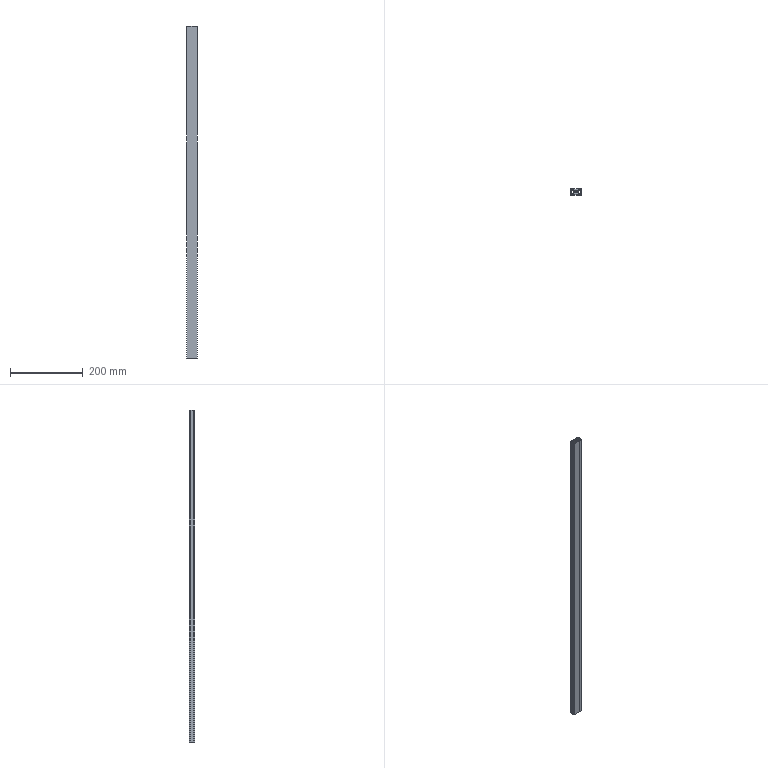Part | SolidWorks | features BaseBody 1, MoveFace 1 | 1 solid | 53 faces | box 30 x 15 x 910 mm | volume 219464 mm3 | plane 38 | cylinder 15 | commonest cylinder face diameters 1 x6 5 x5 2 x4